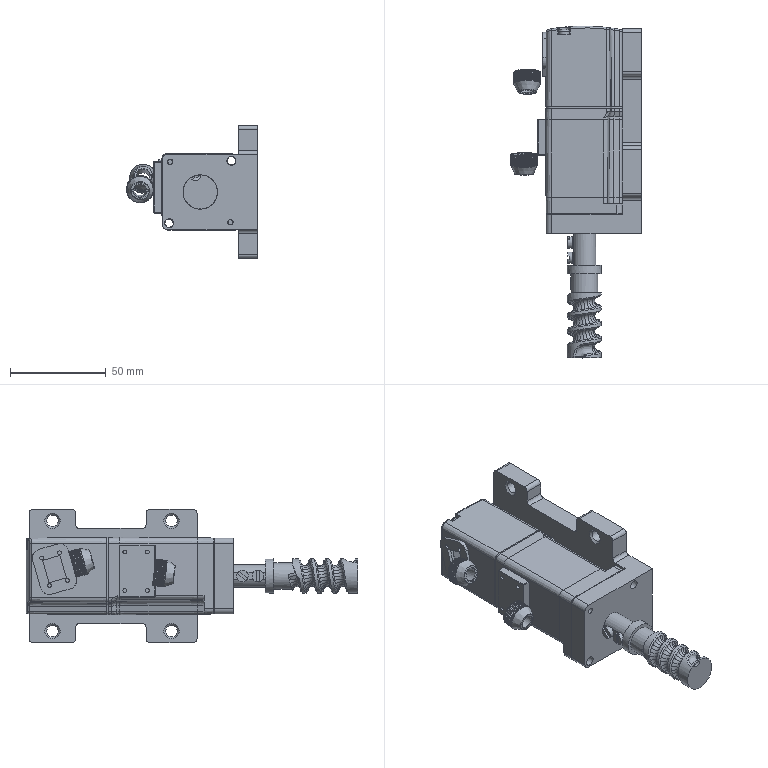Part | NX | features BREP 12 | 10 solids | 1563 faces | box 68.346 x 173.6 x 69.7 mm | volume 178502 mm3 | spline 642 | plane 415 | cone 175 | cylinder 158 | torus 91 | sphere 82 | commonest cylinder face diameters 4 x20 12.2 x12 2 x10 6 x10 2.5 x6 4.002 x6